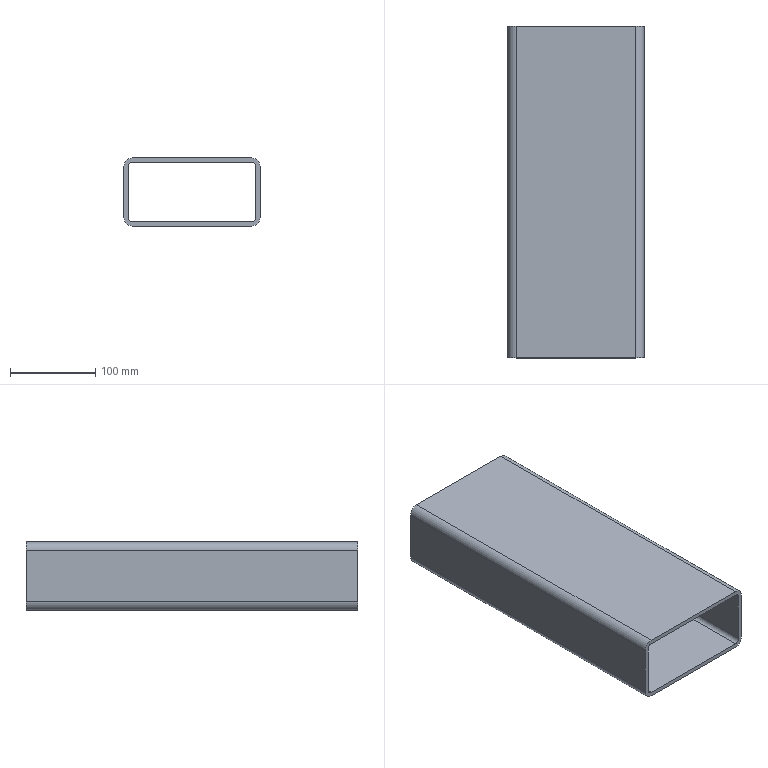Part | SolidWorks | features BaseBody 1 | 1 solid | 18 faces | box 160 x 390 x 80 mm | volume 871892 mm3 | plane 10 | cylinder 8 | commonest cylinder face diameters 10 x4 20 x4
STEP:
#1=CARTESIAN_POINT('',(-70.,195.,40.));
#2=VERTEX_POINT('',#1);
#3=CARTESIAN_POINT('',(-80.,195.,30.));
#4=VERTEX_POINT('',#3);
#5=CARTESIAN_POINT('',(-70.,195.,30.));
#6=DIRECTION('',(0.,-1.,0.));
#7=DIRECTION('',(1.,0.,0.));
#8=AXIS2_PLACEMENT_3D('',#5,#6,#7);
#9=CIRCLE('',#8,10.);
#10=EDGE_CURVE('',#2,#4,#9,.T.);
#11=ORIENTED_EDGE('',*,*,#10,.T.);
#12=CARTESIAN_POINT('',(-80.,-195.,30.));
#13=VERTEX_POINT('',#12);
#14=CARTESIAN_POINT('',(-80.,-195.,30.));
#15=DIRECTION('',(0.,1.,0.));
#16=VECTOR('',#15,1000.);
#17=LINE('',#14,#16);
#18=EDGE_CURVE('',#13,#4,#17,.T.);
#19=ORIENTED_EDGE('',*,*,#18,.F.);
#20=CARTESIAN_POINT('',(-70.,-195.,40.));
#21=VERTEX_POINT('',#20);
#22=CARTESIAN_POINT('',(-70.,-195.,30.));
#23=DIRECTION('',(0.,-1.,0.));
#24=DIRECTION('',(1.,0.,0.));
#25=AXIS2_PLACEMENT_3D('',#22,#23,#24);
#26=CIRCLE('',#25,10.);
#27=EDGE_CURVE('',#21,#13,#26,.T.);
#28=ORIENTED_EDGE('',*,*,#27,.F.);
#29=CARTESIAN_POINT('',(-70.,-195.,40.));
#30=DIRECTION('',(0.,1.,0.));
#31=VECTOR('',#30,1000.);
#32=LINE('',#29,#31);
#33=EDGE_CURVE('',#21,#2,#32,.T.);
#34=ORIENTED_EDGE('',*,*,#33,.T.);
#35=EDGE_LOOP('',(#11,#19,#28,#34));
#36=FACE_OUTER_BOUND('',#35,.T.);
#37=CARTESIAN_POINT('',(-70.,-195.,30.));
#38=DIRECTION('',(0.,1.,0.));
#39=DIRECTION('',(-1.,0.,0.));
#40=AXIS2_PLACEMENT_3D('',#37,#38,#39);
#41=CYLINDRICAL_SURFACE('',#40,10.);
#42=ADVANCED_FACE('',(#36),#41,.T.);
#43=CARTESIAN_POINT('',(-80.,195.,-30.));
#44=VERTEX_POINT('',#43);
#45=CARTESIAN_POINT('',(-80.,195.,30.));
#46=DIRECTION('',(0.,0.,-1.));
#47=VECTOR('',#46,1000.);
#48=LINE('',#45,#47);
#49=EDGE_CURVE('',#4,#44,#48,.T.);
#50=ORIENTED_EDGE('',*,*,#49,.T.);
#51=CARTESIAN_POINT('',(-80.,-195.,-30.));
#52=VERTEX_POINT('',#51);
#53=CARTESIAN_POINT('',(-80.,-195.,-30.));
#54=DIRECTION('',(0.,1.,0.));
#55=VECTOR('',#54,1000.);
#56=LINE('',#53,#55);
#57=EDGE_CURVE('',#52,#44,#56,.T.);
#58=ORIENTED_EDGE('',*,*,#57,.F.);
#59=CARTESIAN_POINT('',(-80.,-195.,30.));
#60=DIRECTION('',(0.,0.,-1.));
#61=VECTOR('',#60,1000.);
#62=LINE('',#59,#61);
#63=EDGE_CURVE('',#13,#52,#62,.T.);
#64=ORIENTED_EDGE('',*,*,#63,.F.);
#65=ORIENTED_EDGE('',*,*,#18,.T.);
#66=EDGE_LOOP('',(#50,#58,#64,#65));
#67=FACE_OUTER_BOUND('',#66,.T.);
#68=CARTESIAN_POINT('',(-80.,-195.,30.));
#69=DIRECTION('',(1.,0.,0.));
#70=DIRECTION('',(0.,0.,-1.));
#71=AXIS2_PLACEMENT_3D('',#68,#69,#70);
#72=PLANE('',#71);
#73=ADVANCED_FACE('',(#67),#72,.F.);
#74=CARTESIAN_POINT('',(-70.,195.,-40.));
#75=VERTEX_POINT('',#74);
#76=CARTESIAN_POINT('',(-70.,195.,-30.));
#77=DIRECTION('',(0.,-1.,0.));
#78=DIRECTION('',(1.,0.,0.));
#79=AXIS2_PLACEMENT_3D('',#76,#77,#78);
#80=CIRCLE('',#79,10.);
#81=EDGE_CURVE('',#44,#75,#80,.T.);
#82=ORIENTED_EDGE('',*,*,#81,.T.);
#83=CARTESIAN_POINT('',(-70.,-195.,-40.));
#84=VERTEX_POINT('',#83);
#85=CARTESIAN_POINT('',(-70.,-195.,-40.));
#86=DIRECTION('',(0.,1.,0.));
#87=VECTOR('',#86,1000.);
#88=LINE('',#85,#87);
#89=EDGE_CURVE('',#84,#75,#88,.T.);
#90=ORIENTED_EDGE('',*,*,#89,.F.);
#91=CARTESIAN_POINT('',(-70.,-195.,-30.));
#92=DIRECTION('',(0.,-1.,0.));
#93=DIRECTION('',(1.,0.,0.));
#94=AXIS2_PLACEMENT_3D('',#91,#92,#93);
#95=CIRCLE('',#94,10.);
#96=EDGE_CURVE('',#52,#84,#95,.T.);
#97=ORIENTED_EDGE('',*,*,#96,.F.);
#98=ORIENTED_EDGE('',*,*,#57,.T.);
#99=EDGE_LOOP('',(#82,#90,#97,#98));
#100=FACE_OUTER_BOUND('',#99,.T.);
#101=CARTESIAN_POINT('',(-70.,-195.,-30.));
#102=DIRECTION('',(0.,1.,0.));
#103=DIRECTION('',(-1.,0.,0.));
#104=AXIS2_PLACEMENT_3D('',#101,#102,#103);
#105=CYLINDRICAL_SURFACE('',#104,10.);
#106=ADVANCED_FACE('',(#100),#105,.T.);
#107=CARTESIAN_POINT('',(70.,195.,-40.));
#108=VERTEX_POINT('',#107);
#109=CARTESIAN_POINT('',(70.,195.,-40.));
#110=DIRECTION('',(1.,0.,0.));
#111=VECTOR('',#110,1000.);
#112=LINE('',#109,#111);
#113=EDGE_CURVE('',#75,#108,#112,.T.);
#114=ORIENTED_EDGE('',*,*,#113,.T.);
#115=CARTESIAN_POINT('',(70.,-195.,-40.));
#116=VERTEX_POINT('',#115);
#117=CARTESIAN_POINT('',(70.,-195.,-40.));
#118=DIRECTION('',(0.,1.,0.));
#119=VECTOR('',#118,1000.);
#120=LINE('',#117,#119);
#121=EDGE_CURVE('',#116,#108,#120,.T.);
#122=ORIENTED_EDGE('',*,*,#121,.F.);
#123=CARTESIAN_POINT('',(70.,-195.,-40.));
#124=DIRECTION('',(1.,0.,0.));
#125=VECTOR('',#124,1000.);
#126=LINE('',#123,#125);
#127=EDGE_CURVE('',#84,#116,#126,.T.);
#128=ORIENTED_EDGE('',*,*,#127,.F.);
#129=ORIENTED_EDGE('',*,*,#89,.T.);
#130=EDGE_LOOP('',(#114,#122,#128,#129));
#131=FACE_OUTER_BOUND('',#130,.T.);
#132=CARTESIAN_POINT('',(70.,-195.,-40.));
#133=DIRECTION('',(0.,0.,1.));
#134=DIRECTION('',(1.,0.,0.));
#135=AXIS2_PLACEMENT_3D('',#132,#133,#134);
#136=PLANE('',#135);
#137=ADVANCED_FACE('',(#131),#136,.F.);
#138=CARTESIAN_POINT('',(80.,195.,-30.));
#139=VERTEX_POINT('',#138);
#140=CARTESIAN_POINT('',(70.,195.,-30.));
#141=DIRECTION('',(0.,-1.,0.));
#142=DIRECTION('',(1.,0.,0.));
#143=AXIS2_PLACEMENT_3D('',#140,#141,#142);
#144=CIRCLE('',#143,10.);
#145=EDGE_CURVE('',#108,#139,#144,.T.);
#146=ORIENTED_EDGE('',*,*,#145,.T.);
#147=CARTESIAN_POINT('',(80.,-195.,-30.));
#148=VERTEX_POINT('',#147);
#149=CARTESIAN_POINT('',(80.,-195.,-30.));
#150=DIRECTION('',(0.,1.,0.));
#151=VECTOR('',#150,1000.);
#152=LINE('',#149,#151);
#153=EDGE_CURVE('',#148,#139,#152,.T.);
#154=ORIENTED_EDGE('',*,*,#153,.F.);
#155=CARTESIAN_POINT('',(70.,-195.,-30.));
#156=DIRECTION('',(0.,-1.,0.));
#157=DIRECTION('',(1.,0.,0.));
#158=AXIS2_PLACEMENT_3D('',#155,#156,#157);
#159=CIRCLE('',#158,10.);
#160=EDGE_CURVE('',#116,#148,#159,.T.);
#161=ORIENTED_EDGE('',*,*,#160,.F.);
#162=ORIENTED_EDGE('',*,*,#121,.T.);
#163=EDGE_LOOP('',(#146,#154,#161,#162));
#164=FACE_OUTER_BOUND('',#163,.T.);
#165=CARTESIAN_POINT('',(70.,-195.,-30.));
#166=DIRECTION('',(0.,1.,0.));
#167=DIRECTION('',(-1.,0.,0.));
#168=AXIS2_PLACEMENT_3D('',#165,#166,#167);
#169=CYLINDRICAL_SURFACE('',#168,10.);
#170=ADVANCED_FACE('',(#164),#169,.T.);
#171=CARTESIAN_POINT('',(80.,195.,30.));
#172=VERTEX_POINT('',#171);
#173=CARTESIAN_POINT('',(80.,195.,-30.));
#174=DIRECTION('',(0.,0.,1.));
#175=VECTOR('',#174,1000.);
#176=LINE('',#173,#175);
#177=EDGE_CURVE('',#139,#172,#176,.T.);
#178=ORIENTED_EDGE('',*,*,#177,.T.);
#179=CARTESIAN_POINT('',(80.,-195.,30.));
#180=VERTEX_POINT('',#179);
#181=CARTESIAN_POINT('',(80.,-195.,30.));
#182=DIRECTION('',(0.,1.,0.));
#183=VECTOR('',#182,1000.);
#184=LINE('',#181,#183);
#185=EDGE_CURVE('',#180,#172,#184,.T.);
#186=ORIENTED_EDGE('',*,*,#185,.F.);
#187=CARTESIAN_POINT('',(80.,-195.,-30.));
#188=DIRECTION('',(0.,0.,1.));
#189=VECTOR('',#188,1000.);
#190=LINE('',#187,#189);
#191=EDGE_CURVE('',#148,#180,#190,.T.);
#192=ORIENTED_EDGE('',*,*,#191,.F.);
#193=ORIENTED_EDGE('',*,*,#153,.T.);
#194=EDGE_LOOP('',(#178,#186,#192,#193));
#195=FACE_OUTER_BOUND('',#194,.T.);
#196=CARTESIAN_POINT('',(80.,-195.,-30.));
#197=DIRECTION('',(-1.,0.,0.));
#198=DIRECTION('',(0.,0.,1.));
#199=AXIS2_PLACEMENT_3D('',#196,#197,#198);
#200=PLANE('',#199);
#201=ADVANCED_FACE('',(#195),#200,.F.);
#202=CARTESIAN_POINT('',(70.,195.,40.));
#203=VERTEX_POINT('',#202);
#204=CARTESIAN_POINT('',(70.,195.,30.));
#205=DIRECTION('',(0.,-1.,0.));
#206=DIRECTION('',(1.,0.,0.));
#207=AXIS2_PLACEMENT_3D('',#204,#205,#206);
#208=CIRCLE('',#207,10.);
#209=EDGE_CURVE('',#172,#203,#208,.T.);
#210=ORIENTED_EDGE('',*,*,#209,.T.);
#211=CARTESIAN_POINT('',(70.,-195.,40.));
#212=VERTEX_POINT('',#211);
#213=CARTESIAN_POINT('',(70.,-195.,40.));
#214=DIRECTION('',(0.,1.,0.));
#215=VECTOR('',#214,1000.);
#216=LINE('',#213,#215);
#217=EDGE_CURVE('',#212,#203,#216,.T.);
#218=ORIENTED_EDGE('',*,*,#217,.F.);
#219=CARTESIAN_POINT('',(70.,-195.,30.));
#220=DIRECTION('',(0.,-1.,0.));
#221=DIRECTION('',(1.,0.,0.));
#222=AXIS2_PLACEMENT_3D('',#219,#220,#221);
#223=CIRCLE('',#222,10.);
#224=EDGE_CURVE('',#180,#212,#223,.T.);
#225=ORIENTED_EDGE('',*,*,#224,.F.);
#226=ORIENTED_EDGE('',*,*,#185,.T.);
#227=EDGE_LOOP('',(#210,#218,#225,#226));
#228=FACE_OUTER_BOUND('',#227,.T.);
#229=CARTESIAN_POINT('',(70.,-195.,30.));
#230=DIRECTION('',(0.,1.,0.));
#231=DIRECTION('',(-1.,0.,0.));
#232=AXIS2_PLACEMENT_3D('',#229,#230,#231);
#233=CYLINDRICAL_SURFACE('',#232,10.);
#234=ADVANCED_FACE('',(#228),#233,.T.);
#235=CARTESIAN_POINT('',(-75.,195.,-30.));
#236=VERTEX_POINT('',#235);
#237=CARTESIAN_POINT('',(-70.,195.,-35.));
#238=VERTEX_POINT('',#237);
#239=CARTESIAN_POINT('',(-70.,195.,-30.));
#240=DIRECTION('',(0.,-1.,0.));
#241=DIRECTION('',(1.,0.,0.));
#242=AXIS2_PLACEMENT_3D('',#239,#240,#241);
#243=CIRCLE('',#242,5.);
#244=EDGE_CURVE('',#236,#238,#243,.T.);
#245=ORIENTED_EDGE('',*,*,#244,.F.);
#246=CARTESIAN_POINT('',(-75.,-195.,-30.));
#247=VERTEX_POINT('',#246);
#248=CARTESIAN_POINT('',(-75.,-195.,-30.));
#249=DIRECTION('',(0.,1.,0.));
#250=VECTOR('',#249,1000.);
#251=LINE('',#248,#250);
#252=EDGE_CURVE('',#247,#236,#251,.T.);
#253=ORIENTED_EDGE('',*,*,#252,.F.);
#254=CARTESIAN_POINT('',(-70.,-195.,-35.));
#255=VERTEX_POINT('',#254);
#256=CARTESIAN_POINT('',(-70.,-195.,-30.));
#257=DIRECTION('',(0.,-1.,0.));
#258=DIRECTION('',(1.,0.,0.));
#259=AXIS2_PLACEMENT_3D('',#256,#257,#258);
#260=CIRCLE('',#259,5.);
#261=EDGE_CURVE('',#247,#255,#260,.T.);
#262=ORIENTED_EDGE('',*,*,#261,.T.);
#263=CARTESIAN_POINT('',(-70.,-195.,-35.));
#264=DIRECTION('',(0.,1.,0.));
#265=VECTOR('',#264,1000.);
#266=LINE('',#263,#265);
#267=EDGE_CURVE('',#255,#238,#266,.T.);
#268=ORIENTED_EDGE('',*,*,#267,.T.);
#269=EDGE_LOOP('',(#245,#253,#262,#268));
#270=FACE_OUTER_BOUND('',#269,.T.);
#271=CARTESIAN_POINT('',(-70.,-195.,-30.));
#272=DIRECTION('',(0.,1.,0.));
#273=DIRECTION('',(-1.,0.,0.));
#274=AXIS2_PLACEMENT_3D('',#271,#272,#273);
#275=CYLINDRICAL_SURFACE('',#274,5.);
#276=ADVANCED_FACE('',(#270),#275,.F.);
#277=CARTESIAN_POINT('',(-75.,195.,30.));
#278=VERTEX_POINT('',#277);
#279=CARTESIAN_POINT('',(-75.,195.,30.));
#280=DIRECTION('',(0.,0.,-1.));
#281=VECTOR('',#280,1000.);
#282=LINE('',#279,#281);
#283=EDGE_CURVE('',#278,#236,#282,.T.);
#284=ORIENTED_EDGE('',*,*,#283,.F.);
#285=CARTESIAN_POINT('',(-75.,-195.,30.));
#286=VERTEX_POINT('',#285);
#287=CARTESIAN_POINT('',(-75.,-195.,30.));
#288=DIRECTION('',(0.,1.,0.));
#289=VECTOR('',#288,1000.);
#290=LINE('',#287,#289);
#291=EDGE_CURVE('',#286,#278,#290,.T.);
#292=ORIENTED_EDGE('',*,*,#291,.F.);
#293=CARTESIAN_POINT('',(-75.,-195.,30.));
#294=DIRECTION('',(0.,0.,-1.));
#295=VECTOR('',#294,1000.);
#296=LINE('',#293,#295);
#297=EDGE_CURVE('',#286,#247,#296,.T.);
#298=ORIENTED_EDGE('',*,*,#297,.T.);
#299=ORIENTED_EDGE('',*,*,#252,.T.);
#300=EDGE_LOOP('',(#284,#292,#298,#299));
#301=FACE_OUTER_BOUND('',#300,.T.);
#302=CARTESIAN_POINT('',(-75.,-195.,30.));
#303=DIRECTION('',(1.,0.,0.));
#304=DIRECTION('',(0.,0.,-1.));
#305=AXIS2_PLACEMENT_3D('',#302,#303,#304);
#306=PLANE('',#305);
#307=ADVANCED_FACE('',(#301),#306,.T.);
#308=CARTESIAN_POINT('',(-70.,195.,35.));
#309=VERTEX_POINT('',#308);
#310=CARTESIAN_POINT('',(-70.,195.,30.));
#311=DIRECTION('',(0.,-1.,0.));
#312=DIRECTION('',(1.,0.,0.));
#313=AXIS2_PLACEMENT_3D('',#310,#311,#312);
#314=CIRCLE('',#313,5.);
#315=EDGE_CURVE('',#309,#278,#314,.T.);
#316=ORIENTED_EDGE('',*,*,#315,.F.);
#317=CARTESIAN_POINT('',(-70.,-195.,35.));
#318=VERTEX_POINT('',#317);
#319=CARTESIAN_POINT('',(-70.,-195.,35.));
#320=DIRECTION('',(0.,1.,0.));
#321=VECTOR('',#320,1000.);
#322=LINE('',#319,#321);
#323=EDGE_CURVE('',#318,#309,#322,.T.);
#324=ORIENTED_EDGE('',*,*,#323,.F.);
#325=CARTESIAN_POINT('',(-70.,-195.,30.));
#326=DIRECTION('',(0.,-1.,0.));
#327=DIRECTION('',(1.,0.,0.));
#328=AXIS2_PLACEMENT_3D('',#325,#326,#327);
#329=CIRCLE('',#328,5.);
#330=EDGE_CURVE('',#318,#286,#329,.T.);
#331=ORIENTED_EDGE('',*,*,#330,.T.);
#332=ORIENTED_EDGE('',*,*,#291,.T.);
#333=EDGE_LOOP('',(#316,#324,#331,#332));
#334=FACE_OUTER_BOUND('',#333,.T.);
#335=CARTESIAN_POINT('',(-70.,-195.,30.));
#336=DIRECTION('',(0.,1.,0.));
#337=DIRECTION('',(-1.,0.,0.));
#338=AXIS2_PLACEMENT_3D('',#335,#336,#337);
#339=CYLINDRICAL_SURFACE('',#338,5.);
#340=ADVANCED_FACE('',(#334),#339,.F.);
#341=CARTESIAN_POINT('',(70.,195.,35.));
#342=VERTEX_POINT('',#341);
#343=CARTESIAN_POINT('',(-70.,195.,35.));
#344=DIRECTION('',(-1.,0.,0.));
#345=VECTOR('',#344,1000.);
#346=LINE('',#343,#345);
#347=EDGE_CURVE('',#342,#309,#346,.T.);
#348=ORIENTED_EDGE('',*,*,#347,.F.);
#349=CARTESIAN_POINT('',(70.,-195.,35.));
#350=VERTEX_POINT('',#349);
#351=CARTESIAN_POINT('',(70.,-195.,35.));
#352=DIRECTION('',(0.,1.,0.));
#353=VECTOR('',#352,1000.);
#354=LINE('',#351,#353);
#355=EDGE_CURVE('',#350,#342,#354,.T.);
#356=ORIENTED_EDGE('',*,*,#355,.F.);
#357=CARTESIAN_POINT('',(-70.,-195.,35.));
#358=DIRECTION('',(-1.,0.,0.));
#359=VECTOR('',#358,1000.);
#360=LINE('',#357,#359);
#361=EDGE_CURVE('',#350,#318,#360,.T.);
#362=ORIENTED_EDGE('',*,*,#361,.T.);
#363=ORIENTED_EDGE('',*,*,#323,.T.);
#364=EDGE_LOOP('',(#348,#356,#362,#363));
#365=FACE_OUTER_BOUND('',#364,.T.);
#366=CARTESIAN_POINT('',(-70.,-195.,35.));
#367=DIRECTION('',(0.,0.,-1.));
#368=DIRECTION('',(-1.,0.,0.));
#369=AXIS2_PLACEMENT_3D('',#366,#367,#368);
#370=PLANE('',#369);
#371=ADVANCED_FACE('',(#365),#370,.T.);
#372=CARTESIAN_POINT('',(75.,195.,30.));
#373=VERTEX_POINT('',#372);
#374=CARTESIAN_POINT('',(70.,195.,30.));
#375=DIRECTION('',(0.,-1.,0.));
#376=DIRECTION('',(1.,0.,0.));
#377=AXIS2_PLACEMENT_3D('',#374,#375,#376);
#378=CIRCLE('',#377,5.);
#379=EDGE_CURVE('',#373,#342,#378,.T.);
#380=ORIENTED_EDGE('',*,*,#379,.F.);
#381=CARTESIAN_POINT('',(75.,-195.,30.));
#382=VERTEX_POINT('',#381);
#383=CARTESIAN_POINT('',(75.,-195.,30.));
#384=DIRECTION('',(0.,1.,0.));
#385=VECTOR('',#384,1000.);
#386=LINE('',#383,#385);
#387=EDGE_CURVE('',#382,#373,#386,.T.);
#388=ORIENTED_EDGE('',*,*,#387,.F.);
#389=CARTESIAN_POINT('',(70.,-195.,30.));
#390=DIRECTION('',(0.,-1.,0.));
#391=DIRECTION('',(1.,0.,0.));
#392=AXIS2_PLACEMENT_3D('',#389,#390,#391);
#393=CIRCLE('',#392,5.);
#394=EDGE_CURVE('',#382,#350,#393,.T.);
#395=ORIENTED_EDGE('',*,*,#394,.T.);
#396=ORIENTED_EDGE('',*,*,#355,.T.);
#397=EDGE_LOOP('',(#380,#388,#395,#396));
#398=FACE_OUTER_BOUND('',#397,.T.);
#399=CARTESIAN_POINT('',(70.,-195.,30.));
#400=DIRECTION('',(0.,1.,0.));
#401=DIRECTION('',(-1.,0.,0.));
#402=AXIS2_PLACEMENT_3D('',#399,#400,#401);
#403=CYLINDRICAL_SURFACE('',#402,5.);
#404=ADVANCED_FACE('',(#398),#403,.F.);
#405=CARTESIAN_POINT('',(75.,195.,-30.));
#406=VERTEX_POINT('',#405);
#407=CARTESIAN_POINT('',(75.,195.,-30.));
#408=DIRECTION('',(0.,0.,1.));
#409=VECTOR('',#408,1000.);
#410=LINE('',#407,#409);
#411=EDGE_CURVE('',#406,#373,#410,.T.);
#412=ORIENTED_EDGE('',*,*,#411,.F.);
#413=CARTESIAN_POINT('',(75.,-195.,-30.));
#414=VERTEX_POINT('',#413);
#415=CARTESIAN_POINT('',(75.,-195.,-30.));
#416=DIRECTION('',(0.,1.,0.));
#417=VECTOR('',#416,1000.);
#418=LINE('',#415,#417);
#419=EDGE_CURVE('',#414,#406,#418,.T.);
#420=ORIENTED_EDGE('',*,*,#419,.F.);
#421=CARTESIAN_POINT('',(75.,-195.,-30.));
#422=DIRECTION('',(0.,0.,1.));
#423=VECTOR('',#422,1000.);
#424=LINE('',#421,#423);
#425=EDGE_CURVE('',#414,#382,#424,.T.);
#426=ORIENTED_EDGE('',*,*,#425,.T.);
#427=ORIENTED_EDGE('',*,*,#387,.T.);
#428=EDGE_LOOP('',(#412,#420,#426,#427));
#429=FACE_OUTER_BOUND('',#428,.T.);
#430=CARTESIAN_POINT('',(75.,-195.,-30.));
#431=DIRECTION('',(-1.,0.,0.));
#432=DIRECTION('',(0.,0.,1.));
#433=AXIS2_PLACEMENT_3D('',#430,#431,#432);
#434=PLANE('',#433);
#435=ADVANCED_FACE('',(#429),#434,.T.);
#436=CARTESIAN_POINT('',(70.,195.,-35.));
#437=VERTEX_POINT('',#436);
#438=CARTESIAN_POINT('',(70.,195.,-30.));
#439=DIRECTION('',(0.,-1.,0.));
#440=DIRECTION('',(1.,0.,0.));
#441=AXIS2_PLACEMENT_3D('',#438,#439,#440);
#442=CIRCLE('',#441,5.);
#443=EDGE_CURVE('',#437,#406,#442,.T.);
#444=ORIENTED_EDGE('',*,*,#443,.F.);
#445=CARTESIAN_POINT('',(70.,-195.,-35.));
#446=VERTEX_POINT('',#445);
#447=CARTESIAN_POINT('',(70.,-195.,-35.));
#448=DIRECTION('',(0.,1.,0.));
#449=VECTOR('',#448,1000.);
#450=LINE('',#447,#449);
#451=EDGE_CURVE('',#446,#437,#450,.T.);
#452=ORIENTED_EDGE('',*,*,#451,.F.);
#453=CARTESIAN_POINT('',(70.,-195.,-30.));
#454=DIRECTION('',(0.,-1.,0.));
#455=DIRECTION('',(1.,0.,0.));
#456=AXIS2_PLACEMENT_3D('',#453,#454,#455);
#457=CIRCLE('',#456,5.);
#458=EDGE_CURVE('',#446,#414,#457,.T.);
#459=ORIENTED_EDGE('',*,*,#458,.T.);
#460=ORIENTED_EDGE('',*,*,#419,.T.);
#461=EDGE_LOOP('',(#444,#452,#459,#460));
#462=FACE_OUTER_BOUND('',#461,.T.);
#463=CARTESIAN_POINT('',(70.,-195.,-30.));
#464=DIRECTION('',(0.,1.,0.));
#465=DIRECTION('',(-1.,0.,0.));
#466=AXIS2_PLACEMENT_3D('',#463,#464,#465);
#467=CYLINDRICAL_SURFACE('',#466,5.);
#468=ADVANCED_FACE('',(#462),#467,.F.);
#469=CARTESIAN_POINT('',(70.,195.,-35.));
#470=DIRECTION('',(1.,0.,0.));
#471=VECTOR('',#470,1000.);
#472=LINE('',#469,#471);
#473=EDGE_CURVE('',#238,#437,#472,.T.);
#474=ORIENTED_EDGE('',*,*,#473,.F.);
#475=ORIENTED_EDGE('',*,*,#267,.F.);
#476=CARTESIAN_POINT('',(70.,-195.,-35.));
#477=DIRECTION('',(1.,0.,0.));
#478=VECTOR('',#477,1000.);
#479=LINE('',#476,#478);
#480=EDGE_CURVE('',#255,#446,#479,.T.);
#481=ORIENTED_EDGE('',*,*,#480,.T.);
#482=ORIENTED_EDGE('',*,*,#451,.T.);
#483=EDGE_LOOP('',(#474,#475,#481,#482));
#484=FACE_OUTER_BOUND('',#483,.T.);
#485=CARTESIAN_POINT('',(70.,-195.,-35.));
#486=DIRECTION('',(0.,0.,1.));
#487=DIRECTION('',(1.,0.,0.));
#488=AXIS2_PLACEMENT_3D('',#485,#486,#487);
#489=PLANE('',#488);
#490=ADVANCED_FACE('',(#484),#489,.T.);
#491=CARTESIAN_POINT('',(-70.,195.,40.));
#492=DIRECTION('',(-1.,0.,0.));
#493=VECTOR('',#492,1000.);
#494=LINE('',#491,#493);
#495=EDGE_CURVE('',#203,#2,#494,.T.);
#496=ORIENTED_EDGE('',*,*,#495,.T.);
#497=ORIENTED_EDGE('',*,*,#33,.F.);
#498=CARTESIAN_POINT('',(-70.,-195.,40.));
#499=DIRECTION('',(-1.,0.,0.));
#500=VECTOR('',#499,1000.);
#501=LINE('',#498,#500);
#502=EDGE_CURVE('',#212,#21,#501,.T.);
#503=ORIENTED_EDGE('',*,*,#502,.F.);
#504=ORIENTED_EDGE('',*,*,#217,.T.);
#505=EDGE_LOOP('',(#496,#497,#503,#504));
#506=FACE_OUTER_BOUND('',#505,.T.);
#507=CARTESIAN_POINT('',(-70.,-195.,40.));
#508=DIRECTION('',(0.,0.,-1.));
#509=DIRECTION('',(-1.,0.,0.));
#510=AXIS2_PLACEMENT_3D('',#507,#508,#509);
#511=PLANE('',#510);
#512=ADVANCED_FACE('',(#506),#511,.F.);
#513=ORIENTED_EDGE('',*,*,#261,.F.);
#514=ORIENTED_EDGE('',*,*,#297,.F.);
#515=ORIENTED_EDGE('',*,*,#330,.F.);
#516=ORIENTED_EDGE('',*,*,#361,.F.);
#517=ORIENTED_EDGE('',*,*,#394,.F.);
#518=ORIENTED_EDGE('',*,*,#425,.F.);
#519=ORIENTED_EDGE('',*,*,#458,.F.);
#520=ORIENTED_EDGE('',*,*,#480,.F.);
#521=EDGE_LOOP('',(#513,#514,#515,#516,#517,#518,#519,#520));
#522=FACE_BOUND('',#521,.T.);
#523=ORIENTED_EDGE('',*,*,#27,.T.);
#524=ORIENTED_EDGE('',*,*,#63,.T.);
#525=ORIENTED_EDGE('',*,*,#96,.T.);
#526=ORIENTED_EDGE('',*,*,#127,.T.);
#527=ORIENTED_EDGE('',*,*,#160,.T.);
#528=ORIENTED_EDGE('',*,*,#191,.T.);
#529=ORIENTED_EDGE('',*,*,#224,.T.);
#530=ORIENTED_EDGE('',*,*,#502,.T.);
#531=EDGE_LOOP('',(#523,#524,#525,#526,#527,#528,#529,#530));
#532=FACE_OUTER_BOUND('',#531,.T.);
#533=CARTESIAN_POINT('',(-70.,-195.,30.));
#534=DIRECTION('',(0.,-1.,0.));
#535=DIRECTION('',(1.,0.,0.));
#536=AXIS2_PLACEMENT_3D('',#533,#534,#535);
#537=PLANE('',#536);
#538=ADVANCED_FACE('',(#522,#532),#537,.T.);
#539=ORIENTED_EDGE('',*,*,#244,.T.);
#540=ORIENTED_EDGE('',*,*,#473,.T.);
#541=ORIENTED_EDGE('',*,*,#443,.T.);
#542=ORIENTED_EDGE('',*,*,#411,.T.);
#543=ORIENTED_EDGE('',*,*,#379,.T.);
#544=ORIENTED_EDGE('',*,*,#347,.T.);
#545=ORIENTED_EDGE('',*,*,#315,.T.);
#546=ORIENTED_EDGE('',*,*,#283,.T.);
#547=EDGE_LOOP('',(#539,#540,#541,#542,#543,#544,#545,#546));
#548=FACE_BOUND('',#547,.T.);
#549=ORIENTED_EDGE('',*,*,#10,.F.);
#550=ORIENTED_EDGE('',*,*,#495,.F.);
#551=ORIENTED_EDGE('',*,*,#209,.F.);
#552=ORIENTED_EDGE('',*,*,#177,.F.);
#553=ORIENTED_EDGE('',*,*,#145,.F.);
#554=ORIENTED_EDGE('',*,*,#113,.F.);
#555=ORIENTED_EDGE('',*,*,#81,.F.);
#556=ORIENTED_EDGE('',*,*,#49,.F.);
#557=EDGE_LOOP('',(#549,#550,#551,#552,#553,#554,#555,#556));
#558=FACE_OUTER_BOUND('',#557,.T.);
#559=CARTESIAN_POINT('',(-70.,195.,30.));
#560=DIRECTION('',(0.,-1.,0.));
#561=DIRECTION('',(1.,0.,0.));
#562=AXIS2_PLACEMENT_3D('',#559,#560,#561);
#563=PLANE('',#562);
#564=ADVANCED_FACE('',(#548,#558),#563,.F.);
#565=CLOSED_SHELL('',(#42,#73,#106,#137,#170,#201,#234,#276,#307,#340,#371,#404,#435,#468,#490,#512,#538,#564));
#566=MANIFOLD_SOLID_BREP('',#565);
#567=CARTESIAN_POINT('',(0.,0.,0.));
#568=DIRECTION('',(0.,0.,1.));
#569=DIRECTION('',(1.,0.,0.));
#570=AXIS2_PLACEMENT_3D('',#567,#568,#569);
#571=(LENGTH_UNIT()NAMED_UNIT(*)SI_UNIT(.MILLI.,.METRE.));
#572=UNCERTAINTY_MEASURE_WITH_UNIT(LENGTH_MEASURE(0.00001),#571,'','');
#573=(NAMED_UNIT(*)PLANE_ANGLE_UNIT()SI_UNIT($,.RADIAN.));
#574=(NAMED_UNIT(*)SI_UNIT($,.STERADIAN.)SOLID_ANGLE_UNIT());
#575=(GEOMETRIC_REPRESENTATION_CONTEXT(3)GLOBAL_UNCERTAINTY_ASSIGNED_CONTEXT((#572))GLOBAL_UNIT_ASSIGNED_CONTEXT((#571,#573,#574))REPRESENTATION_CONTEXT('',''));
#576=ADVANCED_BREP_SHAPE_REPRESENTATION('',(#566,#570),#575);